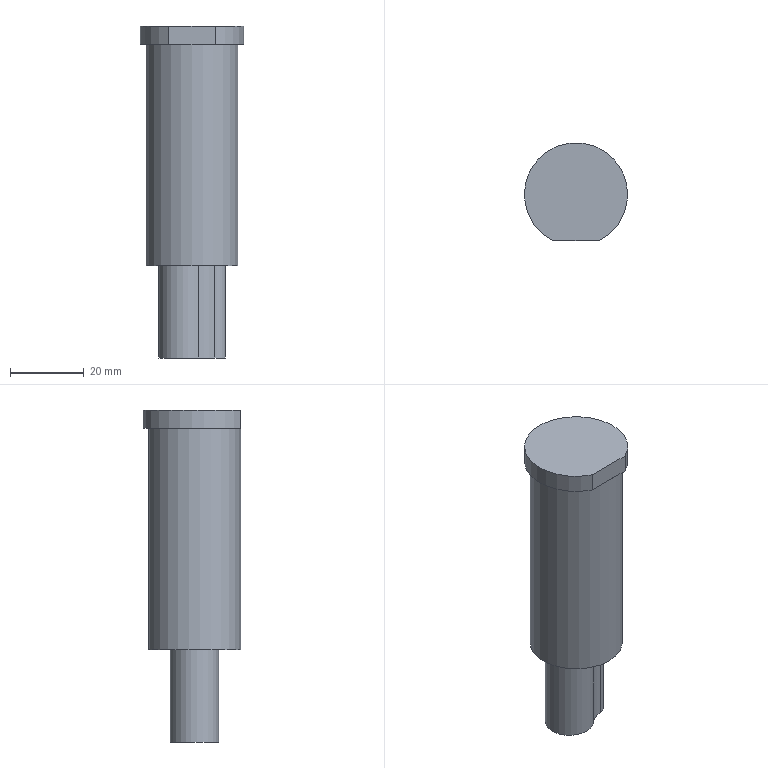Part | NX | features solid 2 | 1 solid | 11 faces | box 28 x 26.5 x 90 mm | volume 36610 mm3 | cylinder 6 | plane 5 | commonest cylinder face diameters 14.2 x2 6.1 x1 13.1 x1 25 x1 28 x1
STEP:
#1=CARTESIAN_POINT('',(-100.353,651.154,41.));
#2=VERTEX_POINT('',#1);
#3=CARTESIAN_POINT('',(-100.353,638.654,41.));
#4=DIRECTION('',(0.,0.,1.));
#5=DIRECTION('',(0.,1.,0.));
#6=AXIS2_PLACEMENT_3D('',#3,#4,#5);
#7=CIRCLE('',#6,12.5);
#8=EDGE_CURVE('',#2,#2,#7,.T.);
#9=ORIENTED_EDGE('',*,*,#8,.F.);
#10=EDGE_LOOP('',(#9));
#11=FACE_BOUND('',#10,.T.);
#12=CARTESIAN_POINT('',(-98.527,633.79,41.));
#13=VERTEX_POINT('',#12);
#14=CARTESIAN_POINT('',(-94.16,635.586,41.));
#15=VERTEX_POINT('',#14);
#16=CARTESIAN_POINT('',(-93.798,628.495,41.));
#17=DIRECTION('',(0.,0.,1.));
#18=DIRECTION('',(1.,0.,0.));
#19=AXIS2_PLACEMENT_3D('',#16,#17,#18);
#20=CIRCLE('',#19,7.1);
#21=EDGE_CURVE('',#13,#15,#20,.F.);
#22=ORIENTED_EDGE('',*,*,#21,.T.);
#23=CARTESIAN_POINT('',(-94.129,641.676,41.));
#24=VERTEX_POINT('',#23);
#25=CARTESIAN_POINT('',(-94.316,638.632,41.));
#26=DIRECTION('',(0.,0.,1.));
#27=DIRECTION('',(1.,0.,0.));
#28=AXIS2_PLACEMENT_3D('',#25,#26,#27);
#29=CIRCLE('',#28,3.05);
#30=EDGE_CURVE('',#15,#24,#29,.T.);
#31=ORIENTED_EDGE('',*,*,#30,.T.);
#32=CARTESIAN_POINT('',(-98.477,643.516,41.));
#33=VERTEX_POINT('',#32);
#34=CARTESIAN_POINT('',(-93.693,648.763,41.));
#35=DIRECTION('',(0.,0.,1.));
#36=DIRECTION('',(1.,0.,0.));
#37=AXIS2_PLACEMENT_3D('',#34,#35,#36);
#38=CIRCLE('',#37,7.1);
#39=EDGE_CURVE('',#24,#33,#38,.F.);
#40=ORIENTED_EDGE('',*,*,#39,.T.);
#41=CARTESIAN_POINT('',(-102.89,638.676,41.));
#42=DIRECTION('',(0.,0.,1.));
#43=DIRECTION('',(1.,0.,0.));
#44=AXIS2_PLACEMENT_3D('',#41,#42,#43);
#45=CIRCLE('',#44,6.55);
#46=EDGE_CURVE('',#33,#13,#45,.T.);
#47=ORIENTED_EDGE('',*,*,#46,.T.);
#48=EDGE_LOOP('',(#22,#31,#40,#47));
#49=FACE_BOUND('',#48,.T.);
#50=CARTESIAN_POINT('',(-100.353,638.654,41.));
#51=DIRECTION('',(0.,0.,1.));
#52=DIRECTION('',(0.,1.,0.));
#53=AXIS2_PLACEMENT_3D('',#50,#51,#52);
#54=PLANE('',#53);
#55=ADVANCED_FACE('',(#11,#49),#54,.F.);
#56=ORIENTED_EDGE('',*,*,#8,.T.);
#57=EDGE_LOOP('',(#56));
#58=FACE_BOUND('',#57,.T.);
#59=CARTESIAN_POINT('',(-100.353,626.154,101.));
#60=VERTEX_POINT('',#59);
#61=CARTESIAN_POINT('',(-100.353,638.654,101.));
#62=DIRECTION('',(0.,0.,1.));
#63=DIRECTION('',(0.,1.,0.));
#64=AXIS2_PLACEMENT_3D('',#61,#62,#63);
#65=CIRCLE('',#64,12.5);
#66=EDGE_CURVE('',#60,#60,#65,.T.);
#67=ORIENTED_EDGE('',*,*,#66,.F.);
#68=EDGE_LOOP('',(#67));
#69=FACE_BOUND('',#68,.T.);
#70=CARTESIAN_POINT('',(-100.353,638.654,106.));
#71=DIRECTION('',(0.,0.,-1.));
#72=DIRECTION('',(0.,-1.,0.));
#73=AXIS2_PLACEMENT_3D('',#70,#71,#72);
#74=CYLINDRICAL_SURFACE('',#73,12.5);
#75=ADVANCED_FACE('',(#58,#69),#74,.T.);
#76=CARTESIAN_POINT('',(-94.048,626.154,101.));
#77=VERTEX_POINT('',#76);
#78=CARTESIAN_POINT('',(-106.658,626.154,101.));
#79=VERTEX_POINT('',#78);
#80=CARTESIAN_POINT('',(-100.353,638.654,101.));
#81=DIRECTION('',(0.,0.,1.));
#82=DIRECTION('',(0.,1.,0.));
#83=AXIS2_PLACEMENT_3D('',#80,#81,#82);
#84=CIRCLE('',#83,14.);
#85=EDGE_CURVE('',#77,#79,#84,.T.);
#86=ORIENTED_EDGE('',*,*,#85,.F.);
#87=CARTESIAN_POINT('',(-100.353,626.154,101.));
#88=DIRECTION('',(-1.,0.,0.));
#89=VECTOR('',#88,1000.);
#90=LINE('',#87,#89);
#91=EDGE_CURVE('',#77,#60,#90,.T.);
#92=ORIENTED_EDGE('',*,*,#91,.T.);
#93=ORIENTED_EDGE('',*,*,#66,.T.);
#94=CARTESIAN_POINT('',(-100.353,626.154,101.));
#95=DIRECTION('',(-1.,0.,0.));
#96=VECTOR('',#95,1000.);
#97=LINE('',#94,#96);
#98=EDGE_CURVE('',#60,#79,#97,.T.);
#99=ORIENTED_EDGE('',*,*,#98,.T.);
#100=EDGE_LOOP('',(#86,#92,#93,#99));
#101=FACE_BOUND('',#100,.T.);
#102=CARTESIAN_POINT('',(-100.353,638.654,101.));
#103=DIRECTION('',(0.,0.,1.));
#104=DIRECTION('',(0.,1.,0.));
#105=AXIS2_PLACEMENT_3D('',#102,#103,#104);
#106=PLANE('',#105);
#107=ADVANCED_FACE('',(#101),#106,.F.);
#108=CARTESIAN_POINT('',(-106.658,626.154,106.));
#109=VERTEX_POINT('',#108);
#110=CARTESIAN_POINT('',(-106.658,626.154,110.));
#111=DIRECTION('',(0.,0.,-1.));
#112=VECTOR('',#111,1000.);
#113=LINE('',#110,#112);
#114=EDGE_CURVE('',#109,#79,#113,.T.);
#115=ORIENTED_EDGE('',*,*,#114,.F.);
#116=CARTESIAN_POINT('',(-94.048,626.154,106.));
#117=VERTEX_POINT('',#116);
#118=CARTESIAN_POINT('',(-100.353,638.654,106.));
#119=DIRECTION('',(0.,0.,1.));
#120=DIRECTION('',(0.,1.,0.));
#121=AXIS2_PLACEMENT_3D('',#118,#119,#120);
#122=CIRCLE('',#121,14.);
#123=EDGE_CURVE('',#117,#109,#122,.T.);
#124=ORIENTED_EDGE('',*,*,#123,.F.);
#125=CARTESIAN_POINT('',(-94.048,626.154,110.));
#126=DIRECTION('',(0.,0.,-1.));
#127=VECTOR('',#126,1000.);
#128=LINE('',#125,#127);
#129=EDGE_CURVE('',#77,#117,#128,.F.);
#130=ORIENTED_EDGE('',*,*,#129,.F.);
#131=ORIENTED_EDGE('',*,*,#85,.T.);
#132=EDGE_LOOP('',(#115,#124,#130,#131));
#133=FACE_BOUND('',#132,.T.);
#134=CARTESIAN_POINT('',(-100.353,638.654,101.));
#135=DIRECTION('',(0.,0.,1.));
#136=DIRECTION('',(0.,1.,0.));
#137=AXIS2_PLACEMENT_3D('',#134,#135,#136);
#138=CYLINDRICAL_SURFACE('',#137,14.);
#139=ADVANCED_FACE('',(#133),#138,.T.);
#140=CARTESIAN_POINT('',(-100.353,626.154,106.));
#141=DIRECTION('',(-1.,0.,0.));
#142=VECTOR('',#141,1000.);
#143=LINE('',#140,#142);
#144=EDGE_CURVE('',#117,#109,#143,.T.);
#145=ORIENTED_EDGE('',*,*,#144,.F.);
#146=ORIENTED_EDGE('',*,*,#123,.T.);
#147=EDGE_LOOP('',(#145,#146));
#148=FACE_BOUND('',#147,.T.);
#149=CARTESIAN_POINT('',(-100.353,638.654,106.));
#150=DIRECTION('',(0.,0.,1.));
#151=DIRECTION('',(0.,1.,0.));
#152=AXIS2_PLACEMENT_3D('',#149,#150,#151);
#153=PLANE('',#152);
#154=ADVANCED_FACE('',(#148),#153,.T.);
#155=ORIENTED_EDGE('',*,*,#129,.T.);
#156=ORIENTED_EDGE('',*,*,#144,.T.);
#157=ORIENTED_EDGE('',*,*,#114,.T.);
#158=ORIENTED_EDGE('',*,*,#98,.F.);
#159=ORIENTED_EDGE('',*,*,#91,.F.);
#160=EDGE_LOOP('',(#155,#156,#157,#158,#159));
#161=FACE_BOUND('',#160,.T.);
#162=CARTESIAN_POINT('',(-106.658,626.154,110.));
#163=DIRECTION('',(0.,1.,0.));
#164=DIRECTION('',(0.,0.,-1.));
#165=AXIS2_PLACEMENT_3D('',#162,#163,#164);
#166=PLANE('',#165);
#167=ADVANCED_FACE('',(#161),#166,.F.);
#168=ORIENTED_EDGE('',*,*,#46,.F.);
#169=CARTESIAN_POINT('',(-98.477,643.516,16.));
#170=VERTEX_POINT('',#169);
#171=CARTESIAN_POINT('',(-98.477,643.516,-80.));
#172=DIRECTION('',(0.,0.,1.));
#173=VECTOR('',#172,1000.);
#174=LINE('',#171,#173);
#175=EDGE_CURVE('',#33,#170,#174,.F.);
#176=ORIENTED_EDGE('',*,*,#175,.T.);
#177=CARTESIAN_POINT('',(-98.527,633.79,16.));
#178=VERTEX_POINT('',#177);
#179=CARTESIAN_POINT('',(-102.89,638.676,16.));
#180=DIRECTION('',(0.,0.,1.));
#181=DIRECTION('',(1.,0.,0.));
#182=AXIS2_PLACEMENT_3D('',#179,#180,#181);
#183=CIRCLE('',#182,6.55);
#184=EDGE_CURVE('',#170,#178,#183,.T.);
#185=ORIENTED_EDGE('',*,*,#184,.T.);
#186=CARTESIAN_POINT('',(-98.527,633.79,-80.));
#187=DIRECTION('',(0.,0.,1.));
#188=VECTOR('',#187,1000.);
#189=LINE('',#186,#188);
#190=EDGE_CURVE('',#178,#13,#189,.T.);
#191=ORIENTED_EDGE('',*,*,#190,.T.);
#192=EDGE_LOOP('',(#168,#176,#185,#191));
#193=FACE_BOUND('',#192,.T.);
#194=CARTESIAN_POINT('',(-102.89,638.676,-80.));
#195=DIRECTION('',(0.,0.,1.));
#196=DIRECTION('',(1.,0.,0.));
#197=AXIS2_PLACEMENT_3D('',#194,#195,#196);
#198=CYLINDRICAL_SURFACE('',#197,6.55);
#199=ADVANCED_FACE('',(#193),#198,.T.);
#200=ORIENTED_EDGE('',*,*,#184,.F.);
#201=CARTESIAN_POINT('',(-94.129,641.676,16.));
#202=VERTEX_POINT('',#201);
#203=CARTESIAN_POINT('',(-93.693,648.763,16.));
#204=DIRECTION('',(0.,0.,1.));
#205=DIRECTION('',(1.,0.,0.));
#206=AXIS2_PLACEMENT_3D('',#203,#204,#205);
#207=CIRCLE('',#206,7.1);
#208=EDGE_CURVE('',#170,#202,#207,.T.);
#209=ORIENTED_EDGE('',*,*,#208,.T.);
#210=CARTESIAN_POINT('',(-94.16,635.586,16.));
#211=VERTEX_POINT('',#210);
#212=CARTESIAN_POINT('',(-94.316,638.632,16.));
#213=DIRECTION('',(0.,0.,1.));
#214=DIRECTION('',(1.,0.,0.));
#215=AXIS2_PLACEMENT_3D('',#212,#213,#214);
#216=CIRCLE('',#215,3.05);
#217=EDGE_CURVE('',#211,#202,#216,.T.);
#218=ORIENTED_EDGE('',*,*,#217,.F.);
#219=CARTESIAN_POINT('',(-93.798,628.495,16.));
#220=DIRECTION('',(0.,0.,1.));
#221=DIRECTION('',(1.,0.,0.));
#222=AXIS2_PLACEMENT_3D('',#219,#220,#221);
#223=CIRCLE('',#222,7.1);
#224=EDGE_CURVE('',#211,#178,#223,.T.);
#225=ORIENTED_EDGE('',*,*,#224,.T.);
#226=EDGE_LOOP('',(#200,#209,#218,#225));
#227=FACE_BOUND('',#226,.T.);
#228=CARTESIAN_POINT('',(-97.853,638.654,16.));
#229=DIRECTION('',(0.,0.,1.));
#230=DIRECTION('',(0.,1.,0.));
#231=AXIS2_PLACEMENT_3D('',#228,#229,#230);
#232=PLANE('',#231);
#233=ADVANCED_FACE('',(#227),#232,.F.);
#234=ORIENTED_EDGE('',*,*,#217,.T.);
#235=CARTESIAN_POINT('',(-94.129,641.676,-80.));
#236=DIRECTION('',(0.,0.,1.));
#237=VECTOR('',#236,1000.);
#238=LINE('',#235,#237);
#239=EDGE_CURVE('',#202,#24,#238,.T.);
#240=ORIENTED_EDGE('',*,*,#239,.T.);
#241=ORIENTED_EDGE('',*,*,#30,.F.);
#242=CARTESIAN_POINT('',(-94.16,635.586,-80.));
#243=DIRECTION('',(0.,0.,1.));
#244=VECTOR('',#243,1000.);
#245=LINE('',#242,#244);
#246=EDGE_CURVE('',#15,#211,#245,.F.);
#247=ORIENTED_EDGE('',*,*,#246,.T.);
#248=EDGE_LOOP('',(#234,#240,#241,#247));
#249=FACE_BOUND('',#248,.T.);
#250=CARTESIAN_POINT('',(-94.316,638.632,-80.));
#251=DIRECTION('',(0.,0.,1.));
#252=DIRECTION('',(1.,0.,0.));
#253=AXIS2_PLACEMENT_3D('',#250,#251,#252);
#254=CYLINDRICAL_SURFACE('',#253,3.05);
#255=ADVANCED_FACE('',(#249),#254,.T.);
#256=ORIENTED_EDGE('',*,*,#21,.F.);
#257=ORIENTED_EDGE('',*,*,#190,.F.);
#258=ORIENTED_EDGE('',*,*,#224,.F.);
#259=ORIENTED_EDGE('',*,*,#246,.F.);
#260=EDGE_LOOP('',(#256,#257,#258,#259));
#261=FACE_BOUND('',#260,.T.);
#262=CARTESIAN_POINT('',(-93.798,628.495,-80.));
#263=DIRECTION('',(0.,0.,1.));
#264=DIRECTION('',(1.,0.,0.));
#265=AXIS2_PLACEMENT_3D('',#262,#263,#264);
#266=CYLINDRICAL_SURFACE('',#265,7.1);
#267=ADVANCED_FACE('',(#261),#266,.F.);
#268=ORIENTED_EDGE('',*,*,#208,.F.);
#269=ORIENTED_EDGE('',*,*,#175,.F.);
#270=ORIENTED_EDGE('',*,*,#39,.F.);
#271=ORIENTED_EDGE('',*,*,#239,.F.);
#272=EDGE_LOOP('',(#268,#269,#270,#271));
#273=FACE_BOUND('',#272,.T.);
#274=CARTESIAN_POINT('',(-93.693,648.763,-80.));
#275=DIRECTION('',(0.,0.,-1.));
#276=DIRECTION('',(-1.,0.,0.));
#277=AXIS2_PLACEMENT_3D('',#274,#275,#276);
#278=CYLINDRICAL_SURFACE('',#277,7.1);
#279=ADVANCED_FACE('',(#273),#278,.F.);
#280=CLOSED_SHELL('',(#55,#75,#107,#139,#154,#167,#199,#233,#255,#267,#279));
#281=MANIFOLD_SOLID_BREP('',#280);
#282=(LENGTH_UNIT()NAMED_UNIT(*)SI_UNIT(.MILLI.,.METRE.));
#283=UNCERTAINTY_MEASURE_WITH_UNIT(LENGTH_MEASURE(0.00001),#282,'','');
#284=(NAMED_UNIT(*)PLANE_ANGLE_UNIT()SI_UNIT($,.RADIAN.));
#285=(NAMED_UNIT(*)SI_UNIT($,.STERADIAN.)SOLID_ANGLE_UNIT());
#286=(GEOMETRIC_REPRESENTATION_CONTEXT(3)GLOBAL_UNCERTAINTY_ASSIGNED_CONTEXT((#283))GLOBAL_UNIT_ASSIGNED_CONTEXT((#282,#284,#285))REPRESENTATION_CONTEXT('',''));
#287=ADVANCED_BREP_SHAPE_REPRESENTATION('',(#281),#286);